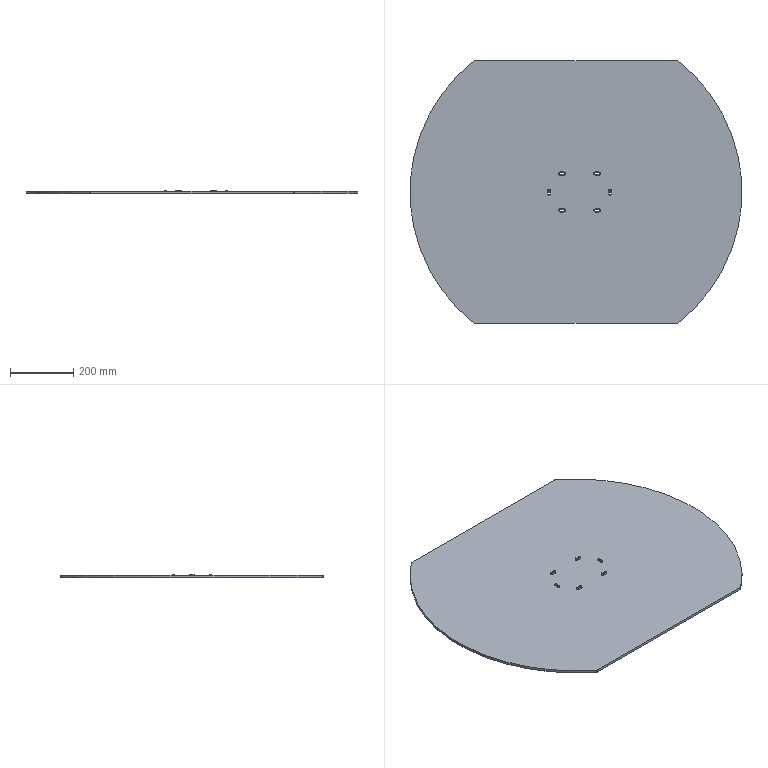Part | NX | features BREP 1 | 1 solid | 104 faces | box 1050 x 830 x 12 mm | volume 6153193 mm3 | plane 50 | cylinder 34 | cone 16 | torus 4 | commonest cylinder face diameters 5.173 x8 8.173 x8 2.4 x4 6.207 x4 10 x4 4.007 x2